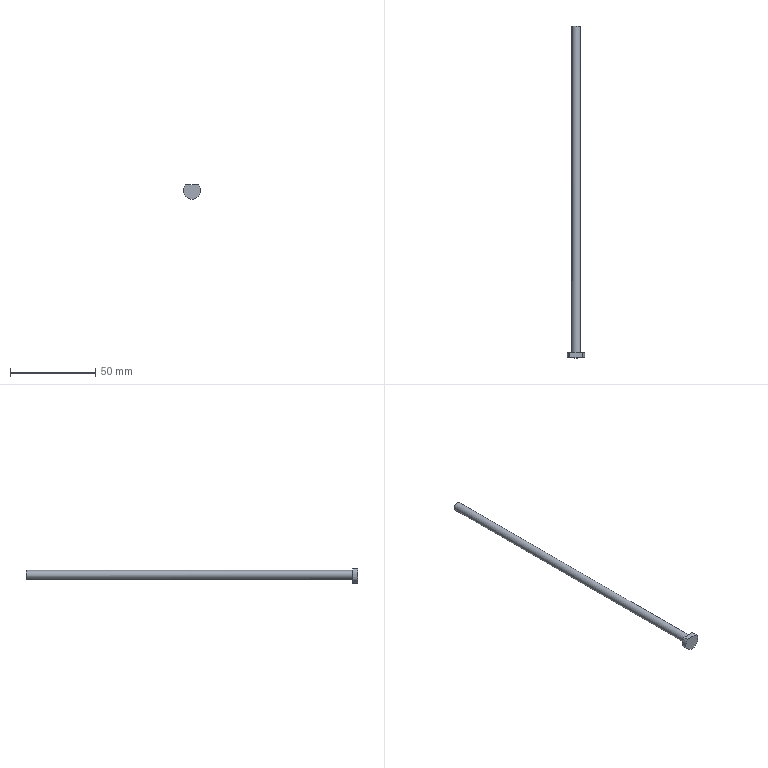Part | STEP file | EJECTION-PIN_id150_x_t | 1 solid | 6 faces | box 10 x 194.406 x 8.5 mm | volume 3970 mm3 | plane 3 | cylinder 3 | commonest cylinder face diameters 5 x1 10 x1 52.427 x1
STEP:
#1=CARTESIAN_POINT('',(-14.919,-220.5,-0.58));
#2=VERTEX_POINT('',#1);
#3=CARTESIAN_POINT('',(-22.061,-220.5,-0.58));
#4=VERTEX_POINT('',#3);
#5=CARTESIAN_POINT('',(-18.49,-220.5,-4.08));
#6=DIRECTION('',(0.,1.,0.));
#7=DIRECTION('',(0.,0.,1.));
#8=AXIS2_PLACEMENT_3D('',#5,#6,#7);
#9=CIRCLE('',#8,5.);
#10=EDGE_CURVE('',#2,#4,#9,.T.);
#11=ORIENTED_EDGE('',*,*,#10,.F.);
#12=CARTESIAN_POINT('',(-22.061,-220.5,-0.58));
#13=DIRECTION('',(1.,0.,0.));
#14=VECTOR('',#13,1.);
#15=LINE('',#12,#14);
#16=EDGE_CURVE('',#4,#2,#15,.T.);
#17=ORIENTED_EDGE('',*,*,#16,.F.);
#18=EDGE_LOOP('',(#11,#17));
#19=FACE_OUTER_BOUND('',#18,.T.);
#20=CARTESIAN_POINT('',(-30.,-220.5,27.));
#21=DIRECTION('',(0.,1.,0.));
#22=DIRECTION('',(0.,0.,1.));
#23=AXIS2_PLACEMENT_3D('',#20,#21,#22);
#24=PLANE('',#23);
#25=ADVANCED_FACE('',(#19),#24,.F.);
#26=CARTESIAN_POINT('',(-22.061,-217.5,-0.58));
#27=VERTEX_POINT('',#26);
#28=CARTESIAN_POINT('',(-22.061,-220.5,-0.58));
#29=DIRECTION('',(0.,1.,0.));
#30=VECTOR('',#29,1.);
#31=LINE('',#28,#30);
#32=EDGE_CURVE('',#4,#27,#31,.T.);
#33=ORIENTED_EDGE('',*,*,#32,.F.);
#34=ORIENTED_EDGE('',*,*,#16,.T.);
#35=CARTESIAN_POINT('',(-14.919,-217.5,-0.58));
#36=VERTEX_POINT('',#35);
#37=CARTESIAN_POINT('',(-14.919,-220.5,-0.58));
#38=DIRECTION('',(0.,-1.,0.));
#39=VECTOR('',#38,1.);
#40=LINE('',#37,#39);
#41=EDGE_CURVE('',#36,#2,#40,.T.);
#42=ORIENTED_EDGE('',*,*,#41,.F.);
#43=CARTESIAN_POINT('',(130.,-217.5,-0.58));
#44=DIRECTION('',(1.,0.,0.));
#45=VECTOR('',#44,1.);
#46=LINE('',#43,#45);
#47=EDGE_CURVE('',#27,#36,#46,.T.);
#48=ORIENTED_EDGE('',*,*,#47,.F.);
#49=EDGE_LOOP('',(#33,#34,#42,#48));
#50=FACE_OUTER_BOUND('',#49,.T.);
#51=CARTESIAN_POINT('',(-22.061,-220.5,-0.58));
#52=DIRECTION('',(0.,0.,1.));
#53=DIRECTION('',(1.,0.,0.));
#54=AXIS2_PLACEMENT_3D('',#51,#52,#53);
#55=PLANE('',#54);
#56=ADVANCED_FACE('',(#50),#55,.T.);
#57=ORIENTED_EDGE('',*,*,#41,.T.);
#58=ORIENTED_EDGE('',*,*,#10,.T.);
#59=ORIENTED_EDGE('',*,*,#32,.T.);
#60=CARTESIAN_POINT('',(-18.49,-217.5,-4.08));
#61=DIRECTION('',(0.,1.,0.));
#62=DIRECTION('',(0.,0.,1.));
#63=AXIS2_PLACEMENT_3D('',#60,#61,#62);
#64=CIRCLE('',#63,5.);
#65=EDGE_CURVE('',#36,#27,#64,.T.);
#66=ORIENTED_EDGE('',*,*,#65,.F.);
#67=EDGE_LOOP('',(#57,#58,#59,#66));
#68=FACE_OUTER_BOUND('',#67,.T.);
#69=CARTESIAN_POINT('',(-18.49,-220.5,-4.08));
#70=DIRECTION('',(0.,1.,0.));
#71=DIRECTION('',(0.,0.,1.));
#72=AXIS2_PLACEMENT_3D('',#69,#70,#71);
#73=CYLINDRICAL_SURFACE('',#72,5.);
#74=ADVANCED_FACE('',(#68),#73,.T.);
#75=CARTESIAN_POINT('',(-20.99,-26.107,-4.08));
#76=VERTEX_POINT('',#75);
#77=CARTESIAN_POINT('',(-20.99,-26.107,-4.08));
#78=CARTESIAN_POINT('',(-20.99,-26.099,-4.359));
#79=CARTESIAN_POINT('',(-20.942,-26.094,-4.641));
#80=CARTESIAN_POINT('',(-20.85,-26.094,-4.904));
#81=CARTESIAN_POINT('',(-20.758,-26.093,-5.167));
#82=CARTESIAN_POINT('',(-20.62,-26.098,-5.418));
#83=CARTESIAN_POINT('',(-20.446,-26.106,-5.636));
#84=CARTESIAN_POINT('',(-20.273,-26.115,-5.855));
#85=CARTESIAN_POINT('',(-20.06,-26.127,-6.046));
#86=CARTESIAN_POINT('',(-19.824,-26.14,-6.194));
#87=CARTESIAN_POINT('',(-19.588,-26.153,-6.343));
#88=CARTESIAN_POINT('',(-19.322,-26.167,-6.454));
#89=CARTESIAN_POINT('',(-19.05,-26.179,-6.516));
#90=CARTESIAN_POINT('',(-18.777,-26.191,-6.579));
#91=CARTESIAN_POINT('',(-18.489,-26.201,-6.596));
#92=CARTESIAN_POINT('',(-18.211,-26.207,-6.564));
#93=CARTESIAN_POINT('',(-17.933,-26.213,-6.533));
#94=CARTESIAN_POINT('',(-17.657,-26.215,-6.453));
#95=CARTESIAN_POINT('',(-17.405,-26.212,-6.332));
#96=CARTESIAN_POINT('',(-17.154,-26.209,-6.211));
#97=CARTESIAN_POINT('',(-16.92,-26.202,-6.045));
#98=CARTESIAN_POINT('',(-16.723,-26.192,-5.849));
#99=CARTESIAN_POINT('',(-16.526,-26.181,-5.652));
#100=CARTESIAN_POINT('',(-16.36,-26.168,-5.418));
#101=CARTESIAN_POINT('',(-16.239,-26.155,-5.167));
#102=CARTESIAN_POINT('',(-16.117,-26.141,-4.915));
#103=CARTESIAN_POINT('',(-16.037,-26.128,-4.638));
#104=CARTESIAN_POINT('',(-16.006,-26.117,-4.36));
#105=CARTESIAN_POINT('',(-15.995,-26.114,-4.267));
#106=CARTESIAN_POINT('',(-15.99,-26.111,-4.174));
#107=CARTESIAN_POINT('',(-15.99,-26.108,-4.08));
#108=CARTESIAN_POINT('',(-15.99,-26.099,-3.801));
#109=CARTESIAN_POINT('',(-16.038,-26.095,-3.519));
#110=CARTESIAN_POINT('',(-16.13,-26.094,-3.256));
#111=CARTESIAN_POINT('',(-16.222,-26.094,-2.992));
#112=CARTESIAN_POINT('',(-16.36,-26.099,-2.742));
#113=CARTESIAN_POINT('',(-16.534,-26.107,-2.523));
#114=CARTESIAN_POINT('',(-16.707,-26.115,-2.305));
#115=CARTESIAN_POINT('',(-16.92,-26.127,-2.114));
#116=CARTESIAN_POINT('',(-17.156,-26.14,-1.966));
#117=CARTESIAN_POINT('',(-17.392,-26.153,-1.817));
#118=CARTESIAN_POINT('',(-17.658,-26.167,-1.706));
#119=CARTESIAN_POINT('',(-17.93,-26.179,-1.643));
#120=CARTESIAN_POINT('',(-18.203,-26.191,-1.581));
#121=CARTESIAN_POINT('',(-18.491,-26.202,-1.564));
#122=CARTESIAN_POINT('',(-18.77,-26.207,-1.596));
#123=CARTESIAN_POINT('',(-19.047,-26.213,-1.627));
#124=CARTESIAN_POINT('',(-19.324,-26.215,-1.707));
#125=CARTESIAN_POINT('',(-19.575,-26.212,-1.828));
#126=CARTESIAN_POINT('',(-19.826,-26.209,-1.949));
#127=CARTESIAN_POINT('',(-20.06,-26.202,-2.115));
#128=CARTESIAN_POINT('',(-20.257,-26.191,-2.311));
#129=CARTESIAN_POINT('',(-20.454,-26.181,-2.508));
#130=CARTESIAN_POINT('',(-20.62,-26.167,-2.742));
#131=CARTESIAN_POINT('',(-20.741,-26.154,-2.993));
#132=CARTESIAN_POINT('',(-20.863,-26.141,-3.245));
#133=CARTESIAN_POINT('',(-20.943,-26.127,-3.522));
#134=CARTESIAN_POINT('',(-20.974,-26.116,-3.8));
#135=CARTESIAN_POINT('',(-20.985,-26.113,-3.893));
#136=CARTESIAN_POINT('',(-20.99,-26.11,-3.986));
#137=CARTESIAN_POINT('',(-20.99,-26.107,-4.08));
#138=B_SPLINE_CURVE_WITH_KNOTS('',3,(#77,#78,#79,#80,#81,#82,#83,#84,#85,#86,#87,#88,#89,#90,#91,#92,#93,#94,#95,#96,#97,#98,#99,#100,#101,#102,#103,#104,#105,#106,#107,#108,#109,#110,#111,#112,#113,#114,#115,#116,#117,#118,#119,#120,#121,#122,#123,#124,#125,#126,#127,#128,#129,#130,#131,#132,#133,#134,#135,#136,#137),.UNSPECIFIED.,.T.,.F.,(1,3,3,3,3,3,3,3,3,3,3,3,3,3,3,3,3,3,3,3,3,3,1),(-0.01772,0.,0.05347,0.1069,0.1604,0.2141,0.2679,0.3215,0.375,0.4285,0.4823,0.5,0.5535,0.6069,0.6604,0.7141,0.7679,0.8215,0.875,0.9285,0.9823,1.,1.053),.UNSPECIFIED.);
#139=EDGE_CURVE('',#76,#76,#138,.T.);
#140=ORIENTED_EDGE('',*,*,#139,.F.);
#141=EDGE_LOOP('',(#140));
#142=FACE_OUTER_BOUND('',#141,.T.);
#143=CARTESIAN_POINT('',(-12.621,0.,-20.64));
#144=DIRECTION('',(0.3338,0.,-0.9426));
#145=DIRECTION('',(-0.9426,0.,-0.3338));
#146=AXIS2_PLACEMENT_3D('',#143,#144,#145);
#147=CYLINDRICAL_SURFACE('',#146,26.213);
#148=ADVANCED_FACE('',(#142),#147,.F.);
#149=CARTESIAN_POINT('',(-18.49,-217.5,-1.58));
#150=VERTEX_POINT('',#149);
#151=CARTESIAN_POINT('',(-18.49,-217.5,-4.08));
#152=DIRECTION('',(0.,1.,0.));
#153=DIRECTION('',(0.,0.,1.));
#154=AXIS2_PLACEMENT_3D('',#151,#152,#153);
#155=CIRCLE('',#154,2.5);
#156=EDGE_CURVE('',#150,#150,#155,.T.);
#157=ORIENTED_EDGE('',*,*,#156,.F.);
#158=EDGE_LOOP('',(#157));
#159=FACE_BOUND('',#158,.T.);
#160=ORIENTED_EDGE('',*,*,#47,.T.);
#161=ORIENTED_EDGE('',*,*,#65,.T.);
#162=EDGE_LOOP('',(#160,#161));
#163=FACE_BOUND('',#162,.T.);
#164=CARTESIAN_POINT('',(130.,-217.5,-52.5));
#165=DIRECTION('',(0.,1.,0.));
#166=DIRECTION('',(0.,0.,1.));
#167=AXIS2_PLACEMENT_3D('',#164,#165,#166);
#168=PLANE('',#167);
#169=ADVANCED_FACE('',(#159,#163),#168,.T.);
#170=ORIENTED_EDGE('',*,*,#139,.T.);
#171=EDGE_LOOP('',(#170));
#172=FACE_BOUND('',#171,.T.);
#173=ORIENTED_EDGE('',*,*,#156,.T.);
#174=EDGE_LOOP('',(#173));
#175=FACE_BOUND('',#174,.T.);
#176=CARTESIAN_POINT('',(-18.49,0.,-4.08));
#177=DIRECTION('',(0.,1.,0.));
#178=DIRECTION('',(0.,0.,1.));
#179=AXIS2_PLACEMENT_3D('',#176,#177,#178);
#180=CYLINDRICAL_SURFACE('',#179,2.5);
#181=ADVANCED_FACE('',(#172,#175),#180,.T.);
#182=CLOSED_SHELL('',(#25,#56,#74,#148,#169,#181));
#183=MANIFOLD_SOLID_BREP('',#182);
#184=(LENGTH_UNIT()NAMED_UNIT(*)SI_UNIT(.MILLI.,.METRE.));
#185=UNCERTAINTY_MEASURE_WITH_UNIT(LENGTH_MEASURE(0.0508),#184,'','');
#186=(NAMED_UNIT(*)PLANE_ANGLE_UNIT()SI_UNIT($,.RADIAN.));
#187=PLANE_ANGLE_MEASURE_WITH_UNIT(PLANE_ANGLE_MEASURE(0.01745),#186);
#188=DIMENSIONAL_EXPONENTS(0.,0.,0.,0.,0.,0.,0.);
#189=(CONVERSION_BASED_UNIT('DEGREE',#187)NAMED_UNIT(#188)PLANE_ANGLE_UNIT());
#190=(NAMED_UNIT(*)SI_UNIT($,.STERADIAN.)SOLID_ANGLE_UNIT());
#191=(GEOMETRIC_REPRESENTATION_CONTEXT(3)GLOBAL_UNCERTAINTY_ASSIGNED_CONTEXT((#185))GLOBAL_UNIT_ASSIGNED_CONTEXT((#184,#189,#190))REPRESENTATION_CONTEXT('',''));
#192=ADVANCED_BREP_SHAPE_REPRESENTATION('',(#183),#191);